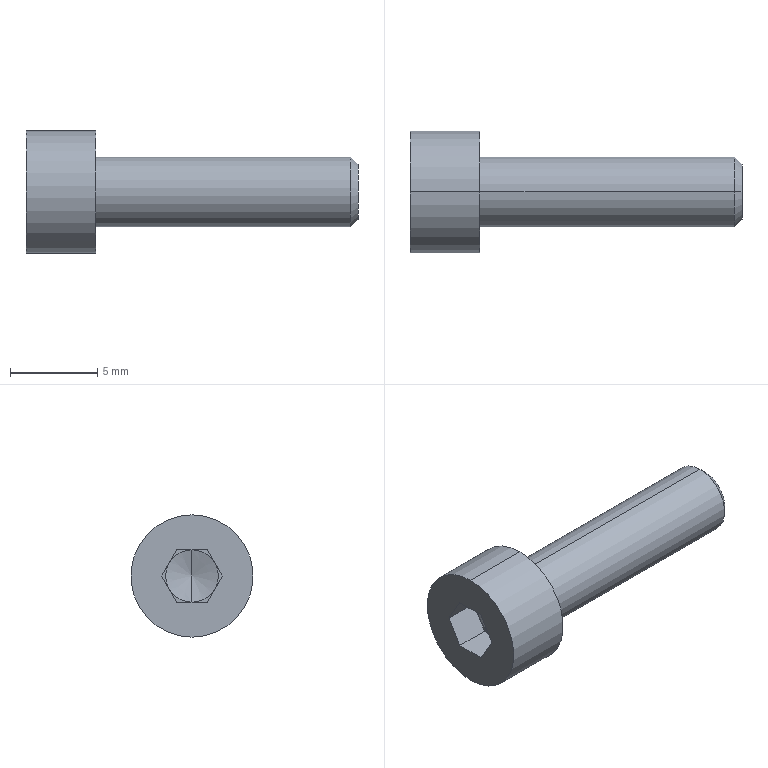Part | SolidWorks | features BaseBody 1 | 1 solid | 23 faces | box 19 x 7 x 7 mm | volume 324.822 mm3 | plane 15 | cylinder 4 | cone 4 | commonest cylinder face diameters 4 x2 7 x2
STEP:
#1=CARTESIAN_POINT('',(0.,0.,-2.));
#2=VERTEX_POINT('',#1);
#3=CARTESIAN_POINT('',(0.,0.,2.));
#4=VERTEX_POINT('',#3);
#5=CARTESIAN_POINT('',(0.,0.,0.));
#6=DIRECTION('',(1.,0.,0.));
#7=DIRECTION('',(0.,0.,-1.));
#8=AXIS2_PLACEMENT_3D('',#5,#6,#7);
#9=CIRCLE('',#8,2.);
#10=EDGE_CURVE('',#2,#4,#9,.T.);
#11=ORIENTED_EDGE('',*,*,#10,.T.);
#12=CARTESIAN_POINT('',(14.571,0.,2.));
#13=VERTEX_POINT('',#12);
#14=CARTESIAN_POINT('',(7.285,0.,2.));
#15=DIRECTION('',(1.,0.,0.));
#16=VECTOR('',#15,1000.);
#17=LINE('',#14,#16);
#18=EDGE_CURVE('',#4,#13,#17,.T.);
#19=ORIENTED_EDGE('',*,*,#18,.T.);
#20=CARTESIAN_POINT('',(14.571,0.,-2.));
#21=VERTEX_POINT('',#20);
#22=CARTESIAN_POINT('',(14.571,0.,0.));
#23=DIRECTION('',(-1.,0.,0.));
#24=DIRECTION('',(0.,0.,-1.));
#25=AXIS2_PLACEMENT_3D('',#22,#23,#24);
#26=CIRCLE('',#25,2.);
#27=EDGE_CURVE('',#13,#21,#26,.T.);
#28=ORIENTED_EDGE('',*,*,#27,.T.);
#29=CARTESIAN_POINT('',(7.285,0.,-2.));
#30=DIRECTION('',(1.,0.,0.));
#31=VECTOR('',#30,1000.);
#32=LINE('',#29,#31);
#33=EDGE_CURVE('',#2,#21,#32,.T.);
#34=ORIENTED_EDGE('',*,*,#33,.F.);
#35=EDGE_LOOP('',(#11,#19,#28,#34));
#36=FACE_OUTER_BOUND('',#35,.T.);
#37=CARTESIAN_POINT('',(7.285,0.,0.));
#38=DIRECTION('',(1.,0.,0.));
#39=DIRECTION('',(0.,0.,-1.));
#40=AXIS2_PLACEMENT_3D('',#37,#38,#39);
#41=CYLINDRICAL_SURFACE('',#40,2.);
#42=ADVANCED_FACE('',(#36),#41,.T.);
#43=CARTESIAN_POINT('',(15.,0.,1.571));
#44=VERTEX_POINT('',#43);
#45=CARTESIAN_POINT('',(15.,0.,-1.571));
#46=VERTEX_POINT('',#45);
#47=CARTESIAN_POINT('',(15.,0.,0.));
#48=DIRECTION('',(-1.,0.,0.));
#49=DIRECTION('',(0.,0.,1.));
#50=AXIS2_PLACEMENT_3D('',#47,#48,#49);
#51=CIRCLE('',#50,1.571);
#52=EDGE_CURVE('',#44,#46,#51,.T.);
#53=ORIENTED_EDGE('',*,*,#52,.T.);
#54=CARTESIAN_POINT('',(14.571,0.,-2.));
#55=DIRECTION('',(-0.7071,0.,-0.7071));
#56=VECTOR('',#55,1000.);
#57=LINE('',#54,#56);
#58=EDGE_CURVE('',#46,#21,#57,.T.);
#59=ORIENTED_EDGE('',*,*,#58,.T.);
#60=ORIENTED_EDGE('',*,*,#27,.F.);
#61=CARTESIAN_POINT('',(14.571,0.,2.));
#62=DIRECTION('',(-0.7071,0.,0.7071));
#63=VECTOR('',#62,1000.);
#64=LINE('',#61,#63);
#65=EDGE_CURVE('',#44,#13,#64,.T.);
#66=ORIENTED_EDGE('',*,*,#65,.F.);
#67=EDGE_LOOP('',(#53,#59,#60,#66));
#68=FACE_OUTER_BOUND('',#67,.T.);
#69=CARTESIAN_POINT('',(14.571,0.,0.));
#70=DIRECTION('',(-1.,0.,0.));
#71=DIRECTION('',(0.,0.,1.));
#72=AXIS2_PLACEMENT_3D('',#69,#70,#71);
#73=CONICAL_SURFACE('',#72,2.,0.7854);
#74=ADVANCED_FACE('',(#68),#73,.T.);
#75=CARTESIAN_POINT('',(-4.,0.,-3.5));
#76=VERTEX_POINT('',#75);
#77=CARTESIAN_POINT('',(-4.,0.,3.5));
#78=VERTEX_POINT('',#77);
#79=CARTESIAN_POINT('',(-4.,0.,0.));
#80=DIRECTION('',(1.,0.,0.));
#81=DIRECTION('',(0.,0.,-1.));
#82=AXIS2_PLACEMENT_3D('',#79,#80,#81);
#83=CIRCLE('',#82,3.5);
#84=EDGE_CURVE('',#76,#78,#83,.T.);
#85=ORIENTED_EDGE('',*,*,#84,.T.);
#86=CARTESIAN_POINT('',(0.,0.,3.5));
#87=VERTEX_POINT('',#86);
#88=CARTESIAN_POINT('',(-2.,0.,3.5));
#89=DIRECTION('',(1.,0.,0.));
#90=VECTOR('',#89,1000.);
#91=LINE('',#88,#90);
#92=EDGE_CURVE('',#78,#87,#91,.T.);
#93=ORIENTED_EDGE('',*,*,#92,.T.);
#94=CARTESIAN_POINT('',(0.,0.,-3.5));
#95=VERTEX_POINT('',#94);
#96=CARTESIAN_POINT('',(0.,0.,0.));
#97=DIRECTION('',(1.,0.,0.));
#98=DIRECTION('',(0.,0.,-1.));
#99=AXIS2_PLACEMENT_3D('',#96,#97,#98);
#100=CIRCLE('',#99,3.5);
#101=EDGE_CURVE('',#95,#87,#100,.T.);
#102=ORIENTED_EDGE('',*,*,#101,.F.);
#103=CARTESIAN_POINT('',(-2.,0.,-3.5));
#104=DIRECTION('',(1.,0.,0.));
#105=VECTOR('',#104,1000.);
#106=LINE('',#103,#105);
#107=EDGE_CURVE('',#76,#95,#106,.T.);
#108=ORIENTED_EDGE('',*,*,#107,.F.);
#109=EDGE_LOOP('',(#85,#93,#102,#108));
#110=FACE_OUTER_BOUND('',#109,.T.);
#111=CARTESIAN_POINT('',(-2.,0.,0.));
#112=DIRECTION('',(1.,0.,0.));
#113=DIRECTION('',(0.,0.,-1.));
#114=AXIS2_PLACEMENT_3D('',#111,#112,#113);
#115=CYLINDRICAL_SURFACE('',#114,3.5);
#116=ADVANCED_FACE('',(#110),#115,.T.);
#117=CARTESIAN_POINT('',(-1.598,0.000000001,0.));
#118=VERTEX_POINT('',#117);
#119=CARTESIAN_POINT('',(-2.,0.,1.5));
#120=VERTEX_POINT('',#119);
#121=CARTESIAN_POINT('',(-2.,0.,1.5));
#122=DIRECTION('',(-0.2588,0.,0.9659));
#123=VECTOR('',#122,1000.);
#124=LINE('',#121,#123);
#125=EDGE_CURVE('',#118,#120,#124,.T.);
#126=ORIENTED_EDGE('',*,*,#125,.F.);
#127=CARTESIAN_POINT('',(-2.,0.,-1.5));
#128=VERTEX_POINT('',#127);
#129=CARTESIAN_POINT('',(-2.,0.,-1.5));
#130=DIRECTION('',(-0.2588,0.,-0.9659));
#131=VECTOR('',#130,1000.);
#132=LINE('',#129,#131);
#133=EDGE_CURVE('',#118,#128,#132,.T.);
#134=ORIENTED_EDGE('',*,*,#133,.T.);
#135=CARTESIAN_POINT('',(-2.,-1.299,-0.75));
#136=VERTEX_POINT('',#135);
#137=CARTESIAN_POINT('',(-2.,0.,0.));
#138=DIRECTION('',(-1.,0.,0.));
#139=DIRECTION('',(0.,0.,1.));
#140=AXIS2_PLACEMENT_3D('',#137,#138,#139);
#141=CIRCLE('',#140,1.5);
#142=EDGE_CURVE('',#128,#136,#141,.T.);
#143=ORIENTED_EDGE('',*,*,#142,.T.);
#144=CARTESIAN_POINT('',(-2.,-1.299,0.75));
#145=VERTEX_POINT('',#144);
#146=CARTESIAN_POINT('',(-2.,0.,0.));
#147=DIRECTION('',(1.,0.,0.));
#148=DIRECTION('',(0.,0.,1.));
#149=AXIS2_PLACEMENT_3D('',#146,#147,#148);
#150=CIRCLE('',#149,1.5);
#151=EDGE_CURVE('',#145,#136,#150,.T.);
#152=ORIENTED_EDGE('',*,*,#151,.F.);
#153=CARTESIAN_POINT('',(-2.,0.,0.));
#154=DIRECTION('',(1.,0.,0.));
#155=DIRECTION('',(0.,0.,1.));
#156=AXIS2_PLACEMENT_3D('',#153,#154,#155);
#157=CIRCLE('',#156,1.5);
#158=EDGE_CURVE('',#120,#145,#157,.T.);
#159=ORIENTED_EDGE('',*,*,#158,.F.);
#160=EDGE_LOOP('',(#126,#134,#143,#152,#159));
#161=FACE_OUTER_BOUND('',#160,.T.);
#162=CARTESIAN_POINT('',(-2.,0.,0.));
#163=DIRECTION('',(-1.,0.,0.));
#164=DIRECTION('',(0.,0.,1.));
#165=AXIS2_PLACEMENT_3D('',#162,#163,#164);
#166=CONICAL_SURFACE('',#165,1.5,1.309);
#167=ADVANCED_FACE('',(#161),#166,.F.);
#168=ORIENTED_EDGE('',*,*,#18,.F.);
#169=CARTESIAN_POINT('',(0.,0.,0.));
#170=DIRECTION('',(1.,0.,0.));
#171=DIRECTION('',(0.,0.,-1.));
#172=AXIS2_PLACEMENT_3D('',#169,#170,#171);
#173=CIRCLE('',#172,2.);
#174=EDGE_CURVE('',#4,#2,#173,.T.);
#175=ORIENTED_EDGE('',*,*,#174,.T.);
#176=ORIENTED_EDGE('',*,*,#33,.T.);
#177=CARTESIAN_POINT('',(14.571,0.,0.));
#178=DIRECTION('',(-1.,0.,0.));
#179=DIRECTION('',(0.,0.,-1.));
#180=AXIS2_PLACEMENT_3D('',#177,#178,#179);
#181=CIRCLE('',#180,2.);
#182=EDGE_CURVE('',#21,#13,#181,.T.);
#183=ORIENTED_EDGE('',*,*,#182,.T.);
#184=EDGE_LOOP('',(#168,#175,#176,#183));
#185=FACE_OUTER_BOUND('',#184,.T.);
#186=CARTESIAN_POINT('',(7.285,0.,0.));
#187=DIRECTION('',(1.,0.,0.));
#188=DIRECTION('',(0.,0.,-1.));
#189=AXIS2_PLACEMENT_3D('',#186,#187,#188);
#190=CYLINDRICAL_SURFACE('',#189,2.);
#191=ADVANCED_FACE('',(#185),#190,.T.);
#192=ORIENTED_EDGE('',*,*,#10,.F.);
#193=ORIENTED_EDGE('',*,*,#174,.F.);
#194=EDGE_LOOP('',(#192,#193));
#195=FACE_BOUND('',#194,.T.);
#196=ORIENTED_EDGE('',*,*,#101,.T.);
#197=CARTESIAN_POINT('',(0.,0.,0.));
#198=DIRECTION('',(1.,0.,0.));
#199=DIRECTION('',(0.,0.,-1.));
#200=AXIS2_PLACEMENT_3D('',#197,#198,#199);
#201=CIRCLE('',#200,3.5);
#202=EDGE_CURVE('',#87,#95,#201,.T.);
#203=ORIENTED_EDGE('',*,*,#202,.T.);
#204=EDGE_LOOP('',(#196,#203));
#205=FACE_OUTER_BOUND('',#204,.T.);
#206=CARTESIAN_POINT('',(0.,2.75,0.));
#207=DIRECTION('',(1.,0.,0.));
#208=DIRECTION('',(0.,0.,-1.));
#209=AXIS2_PLACEMENT_3D('',#206,#207,#208);
#210=PLANE('',#209);
#211=ADVANCED_FACE('',(#195,#205),#210,.T.);
#212=ORIENTED_EDGE('',*,*,#58,.F.);
#213=CARTESIAN_POINT('',(15.,0.,0.));
#214=DIRECTION('',(-1.,0.,0.));
#215=DIRECTION('',(0.,0.,1.));
#216=AXIS2_PLACEMENT_3D('',#213,#214,#215);
#217=CIRCLE('',#216,1.571);
#218=EDGE_CURVE('',#46,#44,#217,.T.);
#219=ORIENTED_EDGE('',*,*,#218,.T.);
#220=ORIENTED_EDGE('',*,*,#65,.T.);
#221=ORIENTED_EDGE('',*,*,#182,.F.);
#222=EDGE_LOOP('',(#212,#219,#220,#221));
#223=FACE_OUTER_BOUND('',#222,.T.);
#224=CARTESIAN_POINT('',(14.571,0.,0.));
#225=DIRECTION('',(-1.,0.,0.));
#226=DIRECTION('',(0.,0.,1.));
#227=AXIS2_PLACEMENT_3D('',#224,#225,#226);
#228=CONICAL_SURFACE('',#227,2.,0.7854);
#229=ADVANCED_FACE('',(#223),#228,.T.);
#230=ORIENTED_EDGE('',*,*,#92,.F.);
#231=CARTESIAN_POINT('',(-4.,0.,0.));
#232=DIRECTION('',(1.,0.,0.));
#233=DIRECTION('',(0.,0.,-1.));
#234=AXIS2_PLACEMENT_3D('',#231,#232,#233);
#235=CIRCLE('',#234,3.5);
#236=EDGE_CURVE('',#78,#76,#235,.T.);
#237=ORIENTED_EDGE('',*,*,#236,.T.);
#238=ORIENTED_EDGE('',*,*,#107,.T.);
#239=ORIENTED_EDGE('',*,*,#202,.F.);
#240=EDGE_LOOP('',(#230,#237,#238,#239));
#241=FACE_OUTER_BOUND('',#240,.T.);
#242=CARTESIAN_POINT('',(-2.,0.,0.));
#243=DIRECTION('',(1.,0.,0.));
#244=DIRECTION('',(0.,0.,-1.));
#245=AXIS2_PLACEMENT_3D('',#242,#243,#244);
#246=CYLINDRICAL_SURFACE('',#245,3.5);
#247=ADVANCED_FACE('',(#241),#246,.T.);
#248=ORIENTED_EDGE('',*,*,#52,.F.);
#249=ORIENTED_EDGE('',*,*,#218,.F.);
#250=EDGE_LOOP('',(#248,#249));
#251=FACE_OUTER_BOUND('',#250,.T.);
#252=CARTESIAN_POINT('',(15.,0.7853,0.));
#253=DIRECTION('',(1.,0.,0.));
#254=DIRECTION('',(0.,0.,-1.));
#255=AXIS2_PLACEMENT_3D('',#252,#253,#254);
#256=PLANE('',#255);
#257=ADVANCED_FACE('',(#251),#256,.T.);
#258=ORIENTED_EDGE('',*,*,#84,.F.);
#259=ORIENTED_EDGE('',*,*,#236,.F.);
#260=EDGE_LOOP('',(#258,#259));
#261=FACE_OUTER_BOUND('',#260,.T.);
#262=CARTESIAN_POINT('',(-4.,0.866,-1.5));
#263=VERTEX_POINT('',#262);
#264=CARTESIAN_POINT('',(-4.,1.732,0.));
#265=VERTEX_POINT('',#264);
#266=CARTESIAN_POINT('',(-4.,1.732,0.));
#267=DIRECTION('',(0.,0.5,0.866));
#268=VECTOR('',#267,1000.);
#269=LINE('',#266,#268);
#270=EDGE_CURVE('',#263,#265,#269,.T.);
#271=ORIENTED_EDGE('',*,*,#270,.T.);
#272=CARTESIAN_POINT('',(-4.,0.866,1.5));
#273=VERTEX_POINT('',#272);
#274=CARTESIAN_POINT('',(-4.,1.732,0.));
#275=DIRECTION('',(0.,-0.5,0.866));
#276=VECTOR('',#275,1000.);
#277=LINE('',#274,#276);
#278=EDGE_CURVE('',#265,#273,#277,.T.);
#279=ORIENTED_EDGE('',*,*,#278,.T.);
#280=CARTESIAN_POINT('',(-4.,-0.866,1.5));
#281=VERTEX_POINT('',#280);
#282=CARTESIAN_POINT('',(-4.,-0.866,1.5));
#283=DIRECTION('',(0.,-1.,0.));
#284=VECTOR('',#283,1000.);
#285=LINE('',#282,#284);
#286=EDGE_CURVE('',#273,#281,#285,.T.);
#287=ORIENTED_EDGE('',*,*,#286,.T.);
#288=CARTESIAN_POINT('',(-4.,-1.732,0.));
#289=VERTEX_POINT('',#288);
#290=CARTESIAN_POINT('',(-4.,-1.732,0.));
#291=DIRECTION('',(0.,-0.5,-0.866));
#292=VECTOR('',#291,1000.);
#293=LINE('',#290,#292);
#294=EDGE_CURVE('',#281,#289,#293,.T.);
#295=ORIENTED_EDGE('',*,*,#294,.T.);
#296=CARTESIAN_POINT('',(-4.,-0.866,-1.5));
#297=VERTEX_POINT('',#296);
#298=CARTESIAN_POINT('',(-4.,-0.866,-1.5));
#299=DIRECTION('',(0.,0.5,-0.866));
#300=VECTOR('',#299,1000.);
#301=LINE('',#298,#300);
#302=EDGE_CURVE('',#289,#297,#301,.T.);
#303=ORIENTED_EDGE('',*,*,#302,.T.);
#304=CARTESIAN_POINT('',(-4.,0.866,-1.5));
#305=DIRECTION('',(0.,1.,0.));
#306=VECTOR('',#305,1000.);
#307=LINE('',#304,#306);
#308=EDGE_CURVE('',#297,#263,#307,.T.);
#309=ORIENTED_EDGE('',*,*,#308,.T.);
#310=EDGE_LOOP('',(#271,#279,#287,#295,#303,#309));
#311=FACE_BOUND('',#310,.T.);
#312=CARTESIAN_POINT('',(-4.,1.75,0.));
#313=DIRECTION('',(-1.,0.,0.));
#314=DIRECTION('',(0.,0.,1.));
#315=AXIS2_PLACEMENT_3D('',#312,#313,#314);
#316=PLANE('',#315);
#317=ADVANCED_FACE('',(#261,#311),#316,.T.);
#318=CARTESIAN_POINT('',(-2.,1.732,0.));
#319=VERTEX_POINT('',#318);
#320=CARTESIAN_POINT('',(-4.,1.732,0.));
#321=DIRECTION('',(-1.,0.,0.));
#322=VECTOR('',#321,1000.);
#323=LINE('',#320,#322);
#324=EDGE_CURVE('',#319,#265,#323,.T.);
#325=ORIENTED_EDGE('',*,*,#324,.F.);
#326=CARTESIAN_POINT('',(-2.,1.299,0.75));
#327=VERTEX_POINT('',#326);
#328=CARTESIAN_POINT('',(-2.,0.866,1.5));
#329=DIRECTION('',(0.,0.5,-0.866));
#330=VECTOR('',#329,1000.);
#331=LINE('',#328,#330);
#332=EDGE_CURVE('',#327,#319,#331,.T.);
#333=ORIENTED_EDGE('',*,*,#332,.F.);
#334=CARTESIAN_POINT('',(-2.,0.866,1.5));
#335=VERTEX_POINT('',#334);
#336=CARTESIAN_POINT('',(-2.,0.866,1.5));
#337=DIRECTION('',(0.,0.5,-0.866));
#338=VECTOR('',#337,1000.);
#339=LINE('',#336,#338);
#340=EDGE_CURVE('',#335,#327,#339,.T.);
#341=ORIENTED_EDGE('',*,*,#340,.F.);
#342=CARTESIAN_POINT('',(-4.,0.866,1.5));
#343=DIRECTION('',(1.,0.,0.));
#344=VECTOR('',#343,1000.);
#345=LINE('',#342,#344);
#346=EDGE_CURVE('',#273,#335,#345,.T.);
#347=ORIENTED_EDGE('',*,*,#346,.F.);
#348=ORIENTED_EDGE('',*,*,#278,.F.);
#349=EDGE_LOOP('',(#325,#333,#341,#347,#348));
#350=FACE_OUTER_BOUND('',#349,.T.);
#351=CARTESIAN_POINT('',(-4.,0.866,1.5));
#352=DIRECTION('',(0.,0.866,0.5));
#353=DIRECTION('',(0.,-0.5,0.866));
#354=AXIS2_PLACEMENT_3D('',#351,#352,#353);
#355=PLANE('',#354);
#356=ADVANCED_FACE('',(#350),#355,.F.);
#357=CARTESIAN_POINT('',(-2.,0.866,-1.5));
#358=VERTEX_POINT('',#357);
#359=CARTESIAN_POINT('',(-4.,0.866,-1.5));
#360=DIRECTION('',(-1.,0.,0.));
#361=VECTOR('',#360,1000.);
#362=LINE('',#359,#361);
#363=EDGE_CURVE('',#358,#263,#362,.T.);
#364=ORIENTED_EDGE('',*,*,#363,.F.);
#365=CARTESIAN_POINT('',(-2.,1.299,-0.75));
#366=VERTEX_POINT('',#365);
#367=CARTESIAN_POINT('',(-2.,1.732,0.));
#368=DIRECTION('',(0.,-0.5,-0.866));
#369=VECTOR('',#368,1000.);
#370=LINE('',#367,#369);
#371=EDGE_CURVE('',#366,#358,#370,.T.);
#372=ORIENTED_EDGE('',*,*,#371,.F.);
#373=CARTESIAN_POINT('',(-2.,1.732,0.));
#374=DIRECTION('',(0.,-0.5,-0.866));
#375=VECTOR('',#374,1000.);
#376=LINE('',#373,#375);
#377=EDGE_CURVE('',#319,#366,#376,.T.);
#378=ORIENTED_EDGE('',*,*,#377,.F.);
#379=ORIENTED_EDGE('',*,*,#324,.T.);
#380=ORIENTED_EDGE('',*,*,#270,.F.);
#381=EDGE_LOOP('',(#364,#372,#378,#379,#380));
#382=FACE_OUTER_BOUND('',#381,.T.);
#383=CARTESIAN_POINT('',(-4.,1.732,0.));
#384=DIRECTION('',(0.,0.866,-0.5));
#385=DIRECTION('',(0.,0.5,0.866));
#386=AXIS2_PLACEMENT_3D('',#383,#384,#385);
#387=PLANE('',#386);
#388=ADVANCED_FACE('',(#382),#387,.F.);
#389=ORIENTED_EDGE('',*,*,#332,.T.);
#390=ORIENTED_EDGE('',*,*,#377,.T.);
#391=CARTESIAN_POINT('',(-2.,0.,0.));
#392=DIRECTION('',(1.,0.,0.));
#393=DIRECTION('',(0.,0.,1.));
#394=AXIS2_PLACEMENT_3D('',#391,#392,#393);
#395=CIRCLE('',#394,1.5);
#396=EDGE_CURVE('',#366,#327,#395,.T.);
#397=ORIENTED_EDGE('',*,*,#396,.T.);
#398=EDGE_LOOP('',(#389,#390,#397));
#399=FACE_OUTER_BOUND('',#398,.T.);
#400=CARTESIAN_POINT('',(-2.,0.,0.));
#401=DIRECTION('',(1.,0.,0.));
#402=DIRECTION('',(0.,0.,-1.));
#403=AXIS2_PLACEMENT_3D('',#400,#401,#402);
#404=PLANE('',#403);
#405=ADVANCED_FACE('',(#399),#404,.F.);
#406=CARTESIAN_POINT('',(-2.,0.,1.5));
#407=DIRECTION('',(0.,-1.,0.));
#408=VECTOR('',#407,1000.);
#409=LINE('',#406,#408);
#410=EDGE_CURVE('',#335,#120,#409,.T.);
#411=ORIENTED_EDGE('',*,*,#410,.F.);
#412=ORIENTED_EDGE('',*,*,#340,.T.);
#413=CARTESIAN_POINT('',(-2.,0.,0.));
#414=DIRECTION('',(-1.,0.,0.));
#415=DIRECTION('',(0.,0.,1.));
#416=AXIS2_PLACEMENT_3D('',#413,#414,#415);
#417=CIRCLE('',#416,1.5);
#418=EDGE_CURVE('',#120,#327,#417,.T.);
#419=ORIENTED_EDGE('',*,*,#418,.F.);
#420=EDGE_LOOP('',(#411,#412,#419));
#421=FACE_OUTER_BOUND('',#420,.T.);
#422=CARTESIAN_POINT('',(-2.,0.,0.));
#423=DIRECTION('',(1.,0.,0.));
#424=DIRECTION('',(0.,0.,-1.));
#425=AXIS2_PLACEMENT_3D('',#422,#423,#424);
#426=PLANE('',#425);
#427=ADVANCED_FACE('',(#421),#426,.F.);
#428=ORIENTED_EDGE('',*,*,#346,.T.);
#429=ORIENTED_EDGE('',*,*,#410,.T.);
#430=CARTESIAN_POINT('',(-2.,-0.866,1.5));
#431=VERTEX_POINT('',#430);
#432=CARTESIAN_POINT('',(-2.,-0.866,1.5));
#433=DIRECTION('',(0.,1.,0.));
#434=VECTOR('',#433,1000.);
#435=LINE('',#432,#434);
#436=EDGE_CURVE('',#431,#120,#435,.T.);
#437=ORIENTED_EDGE('',*,*,#436,.F.);
#438=CARTESIAN_POINT('',(-4.,-0.866,1.5));
#439=DIRECTION('',(1.,0.,0.));
#440=VECTOR('',#439,1000.);
#441=LINE('',#438,#440);
#442=EDGE_CURVE('',#281,#431,#441,.T.);
#443=ORIENTED_EDGE('',*,*,#442,.F.);
#444=ORIENTED_EDGE('',*,*,#286,.F.);
#445=EDGE_LOOP('',(#428,#429,#437,#443,#444));
#446=FACE_OUTER_BOUND('',#445,.T.);
#447=CARTESIAN_POINT('',(-4.,-0.866,1.5));
#448=DIRECTION('',(0.,0.,1.));
#449=DIRECTION('',(1.,0.,0.));
#450=AXIS2_PLACEMENT_3D('',#447,#448,#449);
#451=PLANE('',#450);
#452=ADVANCED_FACE('',(#446),#451,.F.);
#453=CARTESIAN_POINT('',(-2.,-0.866,-1.5));
#454=VERTEX_POINT('',#453);
#455=CARTESIAN_POINT('',(-4.,-0.866,-1.5));
#456=DIRECTION('',(-1.,0.,0.));
#457=VECTOR('',#456,1000.);
#458=LINE('',#455,#457);
#459=EDGE_CURVE('',#454,#297,#458,.T.);
#460=ORIENTED_EDGE('',*,*,#459,.F.);
#461=CARTESIAN_POINT('',(-2.,0.866,-1.5));
#462=DIRECTION('',(0.,-1.,0.));
#463=VECTOR('',#462,1000.);
#464=LINE('',#461,#463);
#465=EDGE_CURVE('',#128,#454,#464,.T.);
#466=ORIENTED_EDGE('',*,*,#465,.F.);
#467=CARTESIAN_POINT('',(-2.,0.866,-1.5));
#468=DIRECTION('',(0.,-1.,0.));
#469=VECTOR('',#468,1000.);
#470=LINE('',#467,#469);
#471=EDGE_CURVE('',#358,#128,#470,.T.);
#472=ORIENTED_EDGE('',*,*,#471,.F.);
#473=ORIENTED_EDGE('',*,*,#363,.T.);
#474=ORIENTED_EDGE('',*,*,#308,.F.);
#475=EDGE_LOOP('',(#460,#466,#472,#473,#474));
#476=FACE_OUTER_BOUND('',#475,.T.);
#477=CARTESIAN_POINT('',(-4.,0.866,-1.5));
#478=DIRECTION('',(0.,0.,-1.));
#479=DIRECTION('',(-1.,0.,0.));
#480=AXIS2_PLACEMENT_3D('',#477,#478,#479);
#481=PLANE('',#480);
#482=ADVANCED_FACE('',(#476),#481,.F.);
#483=ORIENTED_EDGE('',*,*,#371,.T.);
#484=ORIENTED_EDGE('',*,*,#471,.T.);
#485=CARTESIAN_POINT('',(-2.,0.,0.));
#486=DIRECTION('',(-1.,0.,0.));
#487=DIRECTION('',(0.,0.,1.));
#488=AXIS2_PLACEMENT_3D('',#485,#486,#487);
#489=CIRCLE('',#488,1.5);
#490=EDGE_CURVE('',#366,#128,#489,.T.);
#491=ORIENTED_EDGE('',*,*,#490,.F.);
#492=EDGE_LOOP('',(#483,#484,#491));
#493=FACE_OUTER_BOUND('',#492,.T.);
#494=CARTESIAN_POINT('',(-2.,0.,0.));
#495=DIRECTION('',(1.,0.,0.));
#496=DIRECTION('',(0.,0.,-1.));
#497=AXIS2_PLACEMENT_3D('',#494,#495,#496);
#498=PLANE('',#497);
#499=ADVANCED_FACE('',(#493),#498,.F.);
#500=ORIENTED_EDGE('',*,*,#133,.F.);
#501=ORIENTED_EDGE('',*,*,#125,.T.);
#502=ORIENTED_EDGE('',*,*,#418,.T.);
#503=ORIENTED_EDGE('',*,*,#396,.F.);
#504=ORIENTED_EDGE('',*,*,#490,.T.);
#505=EDGE_LOOP('',(#500,#501,#502,#503,#504));
#506=FACE_OUTER_BOUND('',#505,.T.);
#507=CARTESIAN_POINT('',(-2.,0.,0.));
#508=DIRECTION('',(-1.,0.,0.));
#509=DIRECTION('',(0.,0.,1.));
#510=AXIS2_PLACEMENT_3D('',#507,#508,#509);
#511=CONICAL_SURFACE('',#510,1.5,1.309);
#512=ADVANCED_FACE('',(#506),#511,.F.);
#513=CARTESIAN_POINT('',(-2.,-0.866,1.5));
#514=DIRECTION('',(0.,-0.5,-0.866));
#515=VECTOR('',#514,1000.);
#516=LINE('',#513,#515);
#517=EDGE_CURVE('',#431,#145,#516,.T.);
#518=ORIENTED_EDGE('',*,*,#517,.F.);
#519=ORIENTED_EDGE('',*,*,#436,.T.);
#520=ORIENTED_EDGE('',*,*,#158,.T.);
#521=EDGE_LOOP('',(#518,#519,#520));
#522=FACE_OUTER_BOUND('',#521,.T.);
#523=CARTESIAN_POINT('',(-2.,0.,0.));
#524=DIRECTION('',(1.,0.,0.));
#525=DIRECTION('',(0.,0.,-1.));
#526=AXIS2_PLACEMENT_3D('',#523,#524,#525);
#527=PLANE('',#526);
#528=ADVANCED_FACE('',(#522),#527,.F.);
#529=ORIENTED_EDGE('',*,*,#442,.T.);
#530=ORIENTED_EDGE('',*,*,#517,.T.);
#531=CARTESIAN_POINT('',(-2.,-1.732,0.));
#532=VERTEX_POINT('',#531);
#533=CARTESIAN_POINT('',(-2.,-1.732,0.));
#534=DIRECTION('',(0.,0.5,0.866));
#535=VECTOR('',#534,1000.);
#536=LINE('',#533,#535);
#537=EDGE_CURVE('',#532,#145,#536,.T.);
#538=ORIENTED_EDGE('',*,*,#537,.F.);
#539=CARTESIAN_POINT('',(-4.,-1.732,0.));
#540=DIRECTION('',(1.,0.,0.));
#541=VECTOR('',#540,1000.);
#542=LINE('',#539,#541);
#543=EDGE_CURVE('',#289,#532,#542,.T.);
#544=ORIENTED_EDGE('',*,*,#543,.F.);
#545=ORIENTED_EDGE('',*,*,#294,.F.);
#546=EDGE_LOOP('',(#529,#530,#538,#544,#545));
#547=FACE_OUTER_BOUND('',#546,.T.);
#548=CARTESIAN_POINT('',(-4.,-1.732,0.));
#549=DIRECTION('',(0.,-0.866,0.5));
#550=DIRECTION('',(0.,-0.5,-0.866));
#551=AXIS2_PLACEMENT_3D('',#548,#549,#550);
#552=PLANE('',#551);
#553=ADVANCED_FACE('',(#547),#552,.F.);
#554=ORIENTED_EDGE('',*,*,#543,.T.);
#555=CARTESIAN_POINT('',(-2.,-0.866,-1.5));
#556=DIRECTION('',(0.,-0.5,0.866));
#557=VECTOR('',#556,1000.);
#558=LINE('',#555,#557);
#559=EDGE_CURVE('',#136,#532,#558,.T.);
#560=ORIENTED_EDGE('',*,*,#559,.F.);
#561=CARTESIAN_POINT('',(-2.,-0.866,-1.5));
#562=DIRECTION('',(0.,-0.5,0.866));
#563=VECTOR('',#562,1000.);
#564=LINE('',#561,#563);
#565=EDGE_CURVE('',#454,#136,#564,.T.);
#566=ORIENTED_EDGE('',*,*,#565,.F.);
#567=ORIENTED_EDGE('',*,*,#459,.T.);
#568=ORIENTED_EDGE('',*,*,#302,.F.);
#569=EDGE_LOOP('',(#554,#560,#566,#567,#568));
#570=FACE_OUTER_BOUND('',#569,.T.);
#571=CARTESIAN_POINT('',(-4.,-0.866,-1.5));
#572=DIRECTION('',(0.,-0.866,-0.5));
#573=DIRECTION('',(0.,0.5,-0.866));
#574=AXIS2_PLACEMENT_3D('',#571,#572,#573);
#575=PLANE('',#574);
#576=ADVANCED_FACE('',(#570),#575,.F.);
#577=ORIENTED_EDGE('',*,*,#465,.T.);
#578=ORIENTED_EDGE('',*,*,#565,.T.);
#579=ORIENTED_EDGE('',*,*,#142,.F.);
#580=EDGE_LOOP('',(#577,#578,#579));
#581=FACE_OUTER_BOUND('',#580,.T.);
#582=CARTESIAN_POINT('',(-2.,0.,0.));
#583=DIRECTION('',(1.,0.,0.));
#584=DIRECTION('',(0.,0.,-1.));
#585=AXIS2_PLACEMENT_3D('',#582,#583,#584);
#586=PLANE('',#585);
#587=ADVANCED_FACE('',(#581),#586,.F.);
#588=ORIENTED_EDGE('',*,*,#559,.T.);
#589=ORIENTED_EDGE('',*,*,#537,.T.);
#590=ORIENTED_EDGE('',*,*,#151,.T.);
#591=EDGE_LOOP('',(#588,#589,#590));
#592=FACE_OUTER_BOUND('',#591,.T.);
#593=CARTESIAN_POINT('',(-2.,0.,0.));
#594=DIRECTION('',(1.,0.,0.));
#595=DIRECTION('',(0.,0.,-1.));
#596=AXIS2_PLACEMENT_3D('',#593,#594,#595);
#597=PLANE('',#596);
#598=ADVANCED_FACE('',(#592),#597,.F.);
#599=CLOSED_SHELL('',(#42,#74,#116,#167,#191,#211,#229,#247,#257,#317,#356,#388,#405,#427,#452,#482,#499,#512,#528,#553,#576,#587,#598));
#600=MANIFOLD_SOLID_BREP('',#599);
#601=CARTESIAN_POINT('',(0.,0.,0.));
#602=DIRECTION('',(0.,0.,1.));
#603=DIRECTION('',(1.,0.,0.));
#604=AXIS2_PLACEMENT_3D('',#601,#602,#603);
#605=(LENGTH_UNIT()NAMED_UNIT(*)SI_UNIT(.MILLI.,.METRE.));
#606=UNCERTAINTY_MEASURE_WITH_UNIT(LENGTH_MEASURE(0.00001),#605,'','');
#607=(NAMED_UNIT(*)PLANE_ANGLE_UNIT()SI_UNIT($,.RADIAN.));
#608=(NAMED_UNIT(*)SI_UNIT($,.STERADIAN.)SOLID_ANGLE_UNIT());
#609=(GEOMETRIC_REPRESENTATION_CONTEXT(3)GLOBAL_UNCERTAINTY_ASSIGNED_CONTEXT((#606))GLOBAL_UNIT_ASSIGNED_CONTEXT((#605,#607,#608))REPRESENTATION_CONTEXT('',''));
#610=ADVANCED_BREP_SHAPE_REPRESENTATION('',(#600,#604),#609);